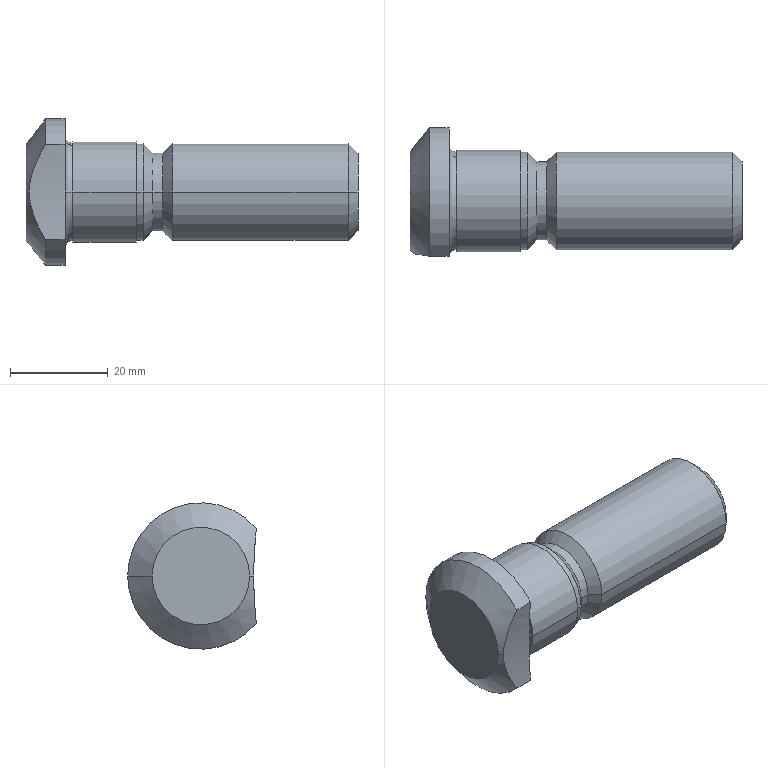Part | STEP file | SCREW_1SHAFTV11 | 1 solid | 28 faces | box 68 x 26.359 x 30 mm | volume 23158 mm3 | cylinder 13 | cone 8 | plane 5 | torus 2 | commonest cylinder face diameters 20 x6 16 x2 20.8 x2 30 x2 183 x1